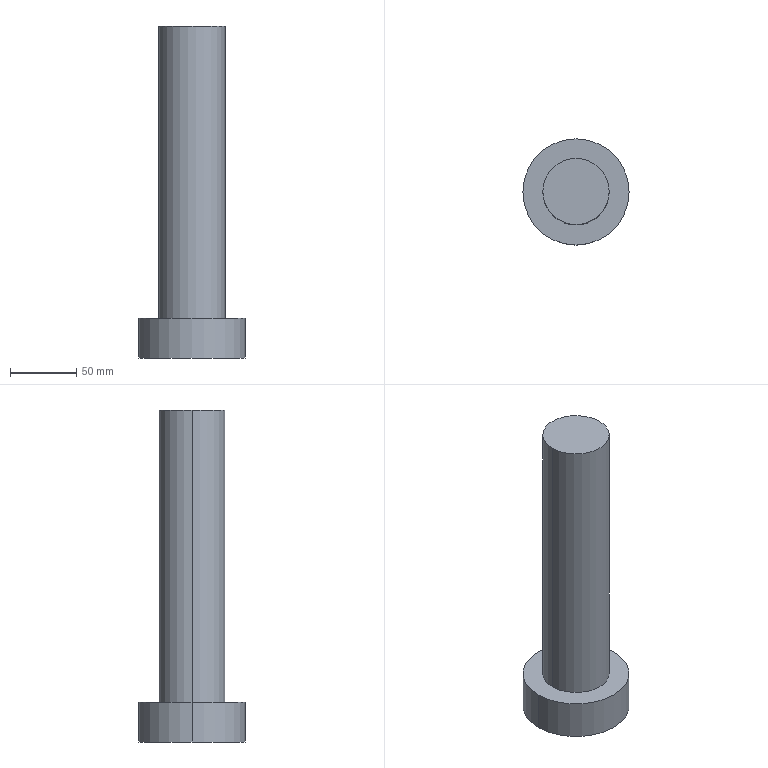Part | SolidWorks | features Extrusion 1, ICE 1 | 1 solid | 7 faces | box 80 x 80 x 250 mm | volume 582765 mm3 | cylinder 4 | plane 3 | commonest cylinder face diameters 50 x2 80 x2
STEP:
#1=CARTESIAN_POINT('',(-40.,0.,-250.));
#2=VERTEX_POINT('',#1);
#3=CARTESIAN_POINT('',(40.,0.,-250.));
#4=VERTEX_POINT('',#3);
#5=CARTESIAN_POINT('',(0.,0.,-250.));
#6=DIRECTION('',(0.,0.,-1.));
#7=DIRECTION('',(-1.,0.,0.));
#8=AXIS2_PLACEMENT_3D('',#5,#6,#7);
#9=CIRCLE('',#8,40.);
#10=EDGE_CURVE('',#2,#4,#9,.T.);
#11=ORIENTED_EDGE('',*,*,#10,.F.);
#12=CARTESIAN_POINT('',(-40.,0.,-220.));
#13=VERTEX_POINT('',#12);
#14=CARTESIAN_POINT('',(-40.,0.,-250.));
#15=DIRECTION('',(0.,0.,1.));
#16=VECTOR('',#15,1000.);
#17=LINE('',#14,#16);
#18=EDGE_CURVE('',#2,#13,#17,.T.);
#19=ORIENTED_EDGE('',*,*,#18,.T.);
#20=CARTESIAN_POINT('',(40.,0.,-220.));
#21=VERTEX_POINT('',#20);
#22=CARTESIAN_POINT('',(0.,0.,-220.));
#23=DIRECTION('',(0.,0.,-1.));
#24=DIRECTION('',(-1.,0.,0.));
#25=AXIS2_PLACEMENT_3D('',#22,#23,#24);
#26=CIRCLE('',#25,40.);
#27=EDGE_CURVE('',#13,#21,#26,.T.);
#28=ORIENTED_EDGE('',*,*,#27,.T.);
#29=CARTESIAN_POINT('',(40.,0.,-250.));
#30=DIRECTION('',(0.,0.,1.));
#31=VECTOR('',#30,1000.);
#32=LINE('',#29,#31);
#33=EDGE_CURVE('',#4,#21,#32,.T.);
#34=ORIENTED_EDGE('',*,*,#33,.F.);
#35=EDGE_LOOP('',(#11,#19,#28,#34));
#36=FACE_OUTER_BOUND('',#35,.T.);
#37=CARTESIAN_POINT('',(0.,0.,-250.));
#38=DIRECTION('',(0.,0.,1.));
#39=DIRECTION('',(1.,0.,0.));
#40=AXIS2_PLACEMENT_3D('',#37,#38,#39);
#41=CYLINDRICAL_SURFACE('',#40,40.);
#42=ADVANCED_FACE('',(#36),#41,.T.);
#43=CARTESIAN_POINT('',(25.,0.,-220.));
#44=VERTEX_POINT('',#43);
#45=CARTESIAN_POINT('',(-25.,0.,-220.));
#46=VERTEX_POINT('',#45);
#47=CARTESIAN_POINT('',(0.,0.,-220.));
#48=DIRECTION('',(0.,0.,1.));
#49=DIRECTION('',(-1.,0.,0.));
#50=AXIS2_PLACEMENT_3D('',#47,#48,#49);
#51=CIRCLE('',#50,25.);
#52=EDGE_CURVE('',#44,#46,#51,.T.);
#53=ORIENTED_EDGE('',*,*,#52,.T.);
#54=CARTESIAN_POINT('',(-25.,0.,0.));
#55=VERTEX_POINT('',#54);
#56=CARTESIAN_POINT('',(-25.,0.,-220.));
#57=DIRECTION('',(0.,0.,1.));
#58=VECTOR('',#57,1000.);
#59=LINE('',#56,#58);
#60=EDGE_CURVE('',#46,#55,#59,.T.);
#61=ORIENTED_EDGE('',*,*,#60,.T.);
#62=CARTESIAN_POINT('',(25.,0.,0.));
#63=VERTEX_POINT('',#62);
#64=CARTESIAN_POINT('',(0.,0.,0.));
#65=DIRECTION('',(0.,0.,1.));
#66=DIRECTION('',(1.,0.,0.));
#67=AXIS2_PLACEMENT_3D('',#64,#65,#66);
#68=CIRCLE('',#67,25.);
#69=EDGE_CURVE('',#63,#55,#68,.T.);
#70=ORIENTED_EDGE('',*,*,#69,.F.);
#71=CARTESIAN_POINT('',(25.,0.,-220.));
#72=DIRECTION('',(0.,0.,1.));
#73=VECTOR('',#72,1000.);
#74=LINE('',#71,#73);
#75=EDGE_CURVE('',#44,#63,#74,.T.);
#76=ORIENTED_EDGE('',*,*,#75,.F.);
#77=EDGE_LOOP('',(#53,#61,#70,#76));
#78=FACE_OUTER_BOUND('',#77,.T.);
#79=CARTESIAN_POINT('',(0.,0.,-220.));
#80=DIRECTION('',(0.,0.,1.));
#81=DIRECTION('',(1.,0.,0.));
#82=AXIS2_PLACEMENT_3D('',#79,#80,#81);
#83=CYLINDRICAL_SURFACE('',#82,25.);
#84=ADVANCED_FACE('',(#78),#83,.T.);
#85=ORIENTED_EDGE('',*,*,#60,.F.);
#86=CARTESIAN_POINT('',(0.,0.,-220.));
#87=DIRECTION('',(0.,0.,1.));
#88=DIRECTION('',(-1.,0.,0.));
#89=AXIS2_PLACEMENT_3D('',#86,#87,#88);
#90=CIRCLE('',#89,25.);
#91=EDGE_CURVE('',#46,#44,#90,.T.);
#92=ORIENTED_EDGE('',*,*,#91,.T.);
#93=ORIENTED_EDGE('',*,*,#75,.T.);
#94=CARTESIAN_POINT('',(0.,0.,0.));
#95=DIRECTION('',(0.,0.,1.));
#96=DIRECTION('',(1.,0.,0.));
#97=AXIS2_PLACEMENT_3D('',#94,#95,#96);
#98=CIRCLE('',#97,25.);
#99=EDGE_CURVE('',#55,#63,#98,.T.);
#100=ORIENTED_EDGE('',*,*,#99,.F.);
#101=EDGE_LOOP('',(#85,#92,#93,#100));
#102=FACE_OUTER_BOUND('',#101,.T.);
#103=CARTESIAN_POINT('',(0.,0.,-220.));
#104=DIRECTION('',(0.,0.,1.));
#105=DIRECTION('',(1.,0.,0.));
#106=AXIS2_PLACEMENT_3D('',#103,#104,#105);
#107=CYLINDRICAL_SURFACE('',#106,25.);
#108=ADVANCED_FACE('',(#102),#107,.T.);
#109=ORIENTED_EDGE('',*,*,#69,.T.);
#110=ORIENTED_EDGE('',*,*,#99,.T.);
#111=EDGE_LOOP('',(#109,#110));
#112=FACE_OUTER_BOUND('',#111,.T.);
#113=CARTESIAN_POINT('',(0.,0.,0.));
#114=DIRECTION('',(0.,0.,1.));
#115=DIRECTION('',(1.,0.,0.));
#116=AXIS2_PLACEMENT_3D('',#113,#114,#115);
#117=PLANE('',#116);
#118=ADVANCED_FACE('',(#112),#117,.T.);
#119=ORIENTED_EDGE('',*,*,#18,.F.);
#120=CARTESIAN_POINT('',(0.,0.,-250.));
#121=DIRECTION('',(0.,0.,-1.));
#122=DIRECTION('',(-1.,0.,0.));
#123=AXIS2_PLACEMENT_3D('',#120,#121,#122);
#124=CIRCLE('',#123,40.);
#125=EDGE_CURVE('',#4,#2,#124,.T.);
#126=ORIENTED_EDGE('',*,*,#125,.F.);
#127=ORIENTED_EDGE('',*,*,#33,.T.);
#128=CARTESIAN_POINT('',(0.,0.,-220.));
#129=DIRECTION('',(0.,0.,-1.));
#130=DIRECTION('',(-1.,0.,0.));
#131=AXIS2_PLACEMENT_3D('',#128,#129,#130);
#132=CIRCLE('',#131,40.);
#133=EDGE_CURVE('',#21,#13,#132,.T.);
#134=ORIENTED_EDGE('',*,*,#133,.T.);
#135=EDGE_LOOP('',(#119,#126,#127,#134));
#136=FACE_OUTER_BOUND('',#135,.T.);
#137=CARTESIAN_POINT('',(0.,0.,-250.));
#138=DIRECTION('',(0.,0.,1.));
#139=DIRECTION('',(1.,0.,0.));
#140=AXIS2_PLACEMENT_3D('',#137,#138,#139);
#141=CYLINDRICAL_SURFACE('',#140,40.);
#142=ADVANCED_FACE('',(#136),#141,.T.);
#143=ORIENTED_EDGE('',*,*,#125,.T.);
#144=ORIENTED_EDGE('',*,*,#10,.T.);
#145=EDGE_LOOP('',(#143,#144));
#146=FACE_OUTER_BOUND('',#145,.T.);
#147=CARTESIAN_POINT('',(0.,0.,-250.));
#148=DIRECTION('',(0.,0.,-1.));
#149=DIRECTION('',(-1.,0.,0.));
#150=AXIS2_PLACEMENT_3D('',#147,#148,#149);
#151=PLANE('',#150);
#152=ADVANCED_FACE('',(#146),#151,.T.);
#153=ORIENTED_EDGE('',*,*,#52,.F.);
#154=ORIENTED_EDGE('',*,*,#91,.F.);
#155=EDGE_LOOP('',(#153,#154));
#156=FACE_BOUND('',#155,.T.);
#157=ORIENTED_EDGE('',*,*,#133,.F.);
#158=ORIENTED_EDGE('',*,*,#27,.F.);
#159=EDGE_LOOP('',(#157,#158));
#160=FACE_OUTER_BOUND('',#159,.T.);
#161=CARTESIAN_POINT('',(0.,0.,-220.));
#162=DIRECTION('',(0.,0.,-1.));
#163=DIRECTION('',(-1.,0.,0.));
#164=AXIS2_PLACEMENT_3D('',#161,#162,#163);
#165=PLANE('',#164);
#166=ADVANCED_FACE('',(#156,#160),#165,.F.);
#167=CLOSED_SHELL('',(#42,#84,#108,#118,#142,#152,#166));
#168=MANIFOLD_SOLID_BREP('',#167);
#169=CARTESIAN_POINT('',(0.,0.,0.));
#170=DIRECTION('',(0.,0.,1.));
#171=DIRECTION('',(1.,0.,0.));
#172=AXIS2_PLACEMENT_3D('',#169,#170,#171);
#173=(LENGTH_UNIT()NAMED_UNIT(*)SI_UNIT(.MILLI.,.METRE.));
#174=UNCERTAINTY_MEASURE_WITH_UNIT(LENGTH_MEASURE(0.00001),#173,'','');
#175=(NAMED_UNIT(*)PLANE_ANGLE_UNIT()SI_UNIT($,.RADIAN.));
#176=(NAMED_UNIT(*)SI_UNIT($,.STERADIAN.)SOLID_ANGLE_UNIT());
#177=(GEOMETRIC_REPRESENTATION_CONTEXT(3)GLOBAL_UNCERTAINTY_ASSIGNED_CONTEXT((#174))GLOBAL_UNIT_ASSIGNED_CONTEXT((#173,#175,#176))REPRESENTATION_CONTEXT('',''));
#178=ADVANCED_BREP_SHAPE_REPRESENTATION('',(#168,#172),#177);